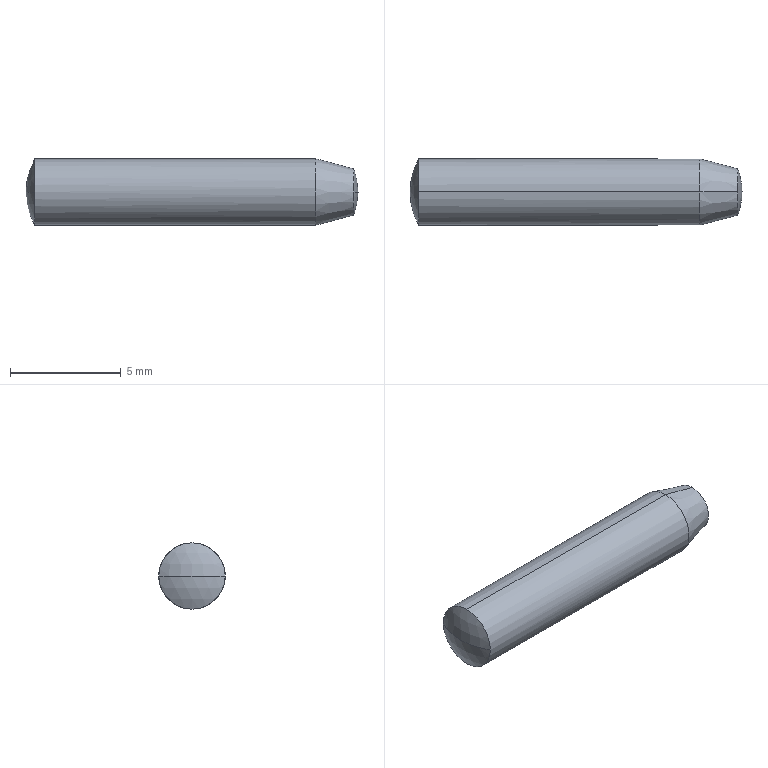Part | NX | features BREP 1 | 1 solid | 8 faces | box 15 x 3 x 3 mm | volume 100.309 mm3 | sphere 4 | cone 2 | cylinder 2 | commonest cylinder face diameters 3 x2
STEP:
#1=CARTESIAN_POINT('',(7.314,-1.04,0.));
#2=VERTEX_POINT('',#1);
#3=CARTESIAN_POINT('',(7.5,0.,0.));
#4=VERTEX_POINT('',#3);
#5=CARTESIAN_POINT('',(4.5,0.,0.));
#6=DIRECTION('',(0.,0.,-1.));
#7=DIRECTION('',(-1.,0.,0.));
#8=AXIS2_PLACEMENT_3D('',#5,#6,#7);
#9=CIRCLE('',#8,3.);
#10=EDGE_CURVE('',#2,#4,#9,.F.);
#11=ORIENTED_EDGE('',*,*,#10,.T.);
#12=CARTESIAN_POINT('',(7.314,1.04,0.));
#13=VERTEX_POINT('',#12);
#14=CARTESIAN_POINT('',(4.5,0.,0.));
#15=DIRECTION('',(0.,0.,1.));
#16=DIRECTION('',(0.,-1.,0.));
#17=AXIS2_PLACEMENT_3D('',#14,#15,#16);
#18=CIRCLE('',#17,3.);
#19=EDGE_CURVE('',#13,#4,#18,.F.);
#20=ORIENTED_EDGE('',*,*,#19,.F.);
#21=CARTESIAN_POINT('',(7.314,0.,1.04));
#22=VERTEX_POINT('',#21);
#23=CARTESIAN_POINT('',(7.314,0.,0.));
#24=DIRECTION('',(-1.,0.,0.));
#25=DIRECTION('',(0.,0.,1.));
#26=AXIS2_PLACEMENT_3D('',#23,#24,#25);
#27=CIRCLE('',#26,1.04);
#28=EDGE_CURVE('',#22,#13,#27,.T.);
#29=ORIENTED_EDGE('',*,*,#28,.F.);
#30=CARTESIAN_POINT('',(7.314,0.,0.));
#31=DIRECTION('',(-1.,0.,0.));
#32=DIRECTION('',(0.,0.,1.));
#33=AXIS2_PLACEMENT_3D('',#30,#31,#32);
#34=CIRCLE('',#33,1.04);
#35=EDGE_CURVE('',#2,#22,#34,.T.);
#36=ORIENTED_EDGE('',*,*,#35,.F.);
#37=EDGE_LOOP('',(#11,#20,#29,#36));
#38=FACE_BOUND('',#37,.T.);
#39=CARTESIAN_POINT('',(4.5,0.,0.));
#40=DIRECTION('',(0.,0.,1.));
#41=DIRECTION('',(0.,1.,0.));
#42=AXIS2_PLACEMENT_3D('',#39,#40,#41);
#43=SPHERICAL_SURFACE('',#42,3.);
#44=ADVANCED_FACE('',(#38),#43,.T.);
#45=ORIENTED_EDGE('',*,*,#28,.T.);
#46=CARTESIAN_POINT('',(7.314,0.,-1.04));
#47=VERTEX_POINT('',#46);
#48=CARTESIAN_POINT('',(7.314,0.,0.));
#49=DIRECTION('',(-1.,0.,0.));
#50=DIRECTION('',(0.,0.,1.));
#51=AXIS2_PLACEMENT_3D('',#48,#49,#50);
#52=CIRCLE('',#51,1.04);
#53=EDGE_CURVE('',#13,#47,#52,.T.);
#54=ORIENTED_EDGE('',*,*,#53,.T.);
#55=CARTESIAN_POINT('',(5.598,0.,-1.5));
#56=VERTEX_POINT('',#55);
#57=CARTESIAN_POINT('',(7.314,0.,-1.04));
#58=DIRECTION('',(-0.9659,0.,-0.2588));
#59=VECTOR('',#58,1000.);
#60=LINE('',#57,#59);
#61=EDGE_CURVE('',#47,#56,#60,.T.);
#62=ORIENTED_EDGE('',*,*,#61,.T.);
#63=CARTESIAN_POINT('',(5.598,0.,1.5));
#64=VERTEX_POINT('',#63);
#65=CARTESIAN_POINT('',(5.598,0.,0.));
#66=DIRECTION('',(-1.,0.,0.));
#67=DIRECTION('',(0.,0.,1.));
#68=AXIS2_PLACEMENT_3D('',#65,#66,#67);
#69=CIRCLE('',#68,1.5);
#70=EDGE_CURVE('',#64,#56,#69,.T.);
#71=ORIENTED_EDGE('',*,*,#70,.F.);
#72=CARTESIAN_POINT('',(7.314,0.,1.04));
#73=DIRECTION('',(-0.9659,0.,0.2588));
#74=VECTOR('',#73,1000.);
#75=LINE('',#72,#74);
#76=EDGE_CURVE('',#22,#64,#75,.T.);
#77=ORIENTED_EDGE('',*,*,#76,.F.);
#78=EDGE_LOOP('',(#45,#54,#62,#71,#77));
#79=FACE_BOUND('',#78,.T.);
#80=CARTESIAN_POINT('',(7.314,0.,0.));
#81=DIRECTION('',(-1.,0.,0.));
#82=DIRECTION('',(0.,0.,-1.));
#83=AXIS2_PLACEMENT_3D('',#80,#81,#82);
#84=CONICAL_SURFACE('',#83,1.04,0.2618);
#85=ADVANCED_FACE('',(#79),#84,.T.);
#86=ORIENTED_EDGE('',*,*,#70,.T.);
#87=CARTESIAN_POINT('',(-7.098,0.,-1.5));
#88=VERTEX_POINT('',#87);
#89=CARTESIAN_POINT('',(7.5,0.,-1.5));
#90=DIRECTION('',(-1.,0.,0.));
#91=VECTOR('',#90,1000.);
#92=LINE('',#89,#91);
#93=EDGE_CURVE('',#56,#88,#92,.T.);
#94=ORIENTED_EDGE('',*,*,#93,.T.);
#95=CARTESIAN_POINT('',(-7.098,1.5,0.));
#96=VERTEX_POINT('',#95);
#97=CARTESIAN_POINT('',(-7.098,0.,0.));
#98=DIRECTION('',(-1.,0.,0.));
#99=DIRECTION('',(0.,0.,1.));
#100=AXIS2_PLACEMENT_3D('',#97,#98,#99);
#101=CIRCLE('',#100,1.5);
#102=EDGE_CURVE('',#96,#88,#101,.T.);
#103=ORIENTED_EDGE('',*,*,#102,.F.);
#104=CARTESIAN_POINT('',(-7.098,0.,1.5));
#105=VERTEX_POINT('',#104);
#106=CARTESIAN_POINT('',(-7.098,0.,0.));
#107=DIRECTION('',(-1.,0.,0.));
#108=DIRECTION('',(0.,0.,1.));
#109=AXIS2_PLACEMENT_3D('',#106,#107,#108);
#110=CIRCLE('',#109,1.5);
#111=EDGE_CURVE('',#105,#96,#110,.T.);
#112=ORIENTED_EDGE('',*,*,#111,.F.);
#113=CARTESIAN_POINT('',(7.5,0.,1.5));
#114=DIRECTION('',(-1.,0.,0.));
#115=VECTOR('',#114,1000.);
#116=LINE('',#113,#115);
#117=EDGE_CURVE('',#64,#105,#116,.T.);
#118=ORIENTED_EDGE('',*,*,#117,.F.);
#119=EDGE_LOOP('',(#86,#94,#103,#112,#118));
#120=FACE_BOUND('',#119,.T.);
#121=CARTESIAN_POINT('',(7.5,0.,0.));
#122=DIRECTION('',(-1.,0.,0.));
#123=DIRECTION('',(0.,0.,-1.));
#124=AXIS2_PLACEMENT_3D('',#121,#122,#123);
#125=CYLINDRICAL_SURFACE('',#124,1.5);
#126=ADVANCED_FACE('',(#120),#125,.T.);
#127=ORIENTED_EDGE('',*,*,#102,.T.);
#128=CARTESIAN_POINT('',(-7.098,-1.5,0.));
#129=VERTEX_POINT('',#128);
#130=CARTESIAN_POINT('',(-7.098,0.,0.));
#131=DIRECTION('',(-1.,0.,0.));
#132=DIRECTION('',(0.,0.,1.));
#133=AXIS2_PLACEMENT_3D('',#130,#131,#132);
#134=CIRCLE('',#133,1.5);
#135=EDGE_CURVE('',#88,#129,#134,.T.);
#136=ORIENTED_EDGE('',*,*,#135,.T.);
#137=CARTESIAN_POINT('',(-7.5,0.,0.));
#138=VERTEX_POINT('',#137);
#139=CARTESIAN_POINT('',(-4.5,0.,0.));
#140=DIRECTION('',(0.,0.,-1.));
#141=DIRECTION('',(0.,1.,0.));
#142=AXIS2_PLACEMENT_3D('',#139,#140,#141);
#143=CIRCLE('',#142,3.);
#144=EDGE_CURVE('',#129,#138,#143,.T.);
#145=ORIENTED_EDGE('',*,*,#144,.T.);
#146=CARTESIAN_POINT('',(-4.5,0.,0.));
#147=DIRECTION('',(0.,0.,1.));
#148=DIRECTION('',(1.,0.,0.));
#149=AXIS2_PLACEMENT_3D('',#146,#147,#148);
#150=CIRCLE('',#149,3.);
#151=EDGE_CURVE('',#96,#138,#150,.T.);
#152=ORIENTED_EDGE('',*,*,#151,.F.);
#153=EDGE_LOOP('',(#127,#136,#145,#152));
#154=FACE_BOUND('',#153,.T.);
#155=CARTESIAN_POINT('',(-4.5,0.,0.));
#156=DIRECTION('',(0.,0.,-1.));
#157=DIRECTION('',(0.,-1.,0.));
#158=AXIS2_PLACEMENT_3D('',#155,#156,#157);
#159=SPHERICAL_SURFACE('',#158,3.);
#160=ADVANCED_FACE('',(#154),#159,.T.);
#161=ORIENTED_EDGE('',*,*,#144,.F.);
#162=CARTESIAN_POINT('',(-7.098,0.,0.));
#163=DIRECTION('',(-1.,0.,0.));
#164=DIRECTION('',(0.,0.,1.));
#165=AXIS2_PLACEMENT_3D('',#162,#163,#164);
#166=CIRCLE('',#165,1.5);
#167=EDGE_CURVE('',#129,#105,#166,.T.);
#168=ORIENTED_EDGE('',*,*,#167,.T.);
#169=ORIENTED_EDGE('',*,*,#111,.T.);
#170=ORIENTED_EDGE('',*,*,#151,.T.);
#171=EDGE_LOOP('',(#161,#168,#169,#170));
#172=FACE_BOUND('',#171,.T.);
#173=CARTESIAN_POINT('',(-4.5,0.,0.));
#174=DIRECTION('',(0.,0.,-1.));
#175=DIRECTION('',(0.,-1.,0.));
#176=AXIS2_PLACEMENT_3D('',#173,#174,#175);
#177=SPHERICAL_SURFACE('',#176,3.);
#178=ADVANCED_FACE('',(#172),#177,.T.);
#179=ORIENTED_EDGE('',*,*,#93,.F.);
#180=CARTESIAN_POINT('',(5.598,0.,0.));
#181=DIRECTION('',(-1.,0.,0.));
#182=DIRECTION('',(0.,0.,1.));
#183=AXIS2_PLACEMENT_3D('',#180,#181,#182);
#184=CIRCLE('',#183,1.5);
#185=EDGE_CURVE('',#56,#64,#184,.T.);
#186=ORIENTED_EDGE('',*,*,#185,.T.);
#187=ORIENTED_EDGE('',*,*,#117,.T.);
#188=ORIENTED_EDGE('',*,*,#167,.F.);
#189=ORIENTED_EDGE('',*,*,#135,.F.);
#190=EDGE_LOOP('',(#179,#186,#187,#188,#189));
#191=FACE_BOUND('',#190,.T.);
#192=CARTESIAN_POINT('',(7.5,0.,0.));
#193=DIRECTION('',(-1.,0.,0.));
#194=DIRECTION('',(0.,0.,-1.));
#195=AXIS2_PLACEMENT_3D('',#192,#193,#194);
#196=CYLINDRICAL_SURFACE('',#195,1.5);
#197=ADVANCED_FACE('',(#191),#196,.T.);
#198=ORIENTED_EDGE('',*,*,#61,.F.);
#199=CARTESIAN_POINT('',(7.314,0.,0.));
#200=DIRECTION('',(-1.,0.,0.));
#201=DIRECTION('',(0.,0.,1.));
#202=AXIS2_PLACEMENT_3D('',#199,#200,#201);
#203=CIRCLE('',#202,1.04);
#204=EDGE_CURVE('',#47,#2,#203,.T.);
#205=ORIENTED_EDGE('',*,*,#204,.T.);
#206=ORIENTED_EDGE('',*,*,#35,.T.);
#207=ORIENTED_EDGE('',*,*,#76,.T.);
#208=ORIENTED_EDGE('',*,*,#185,.F.);
#209=EDGE_LOOP('',(#198,#205,#206,#207,#208));
#210=FACE_BOUND('',#209,.T.);
#211=CARTESIAN_POINT('',(7.314,0.,0.));
#212=DIRECTION('',(-1.,0.,0.));
#213=DIRECTION('',(0.,0.,-1.));
#214=AXIS2_PLACEMENT_3D('',#211,#212,#213);
#215=CONICAL_SURFACE('',#214,1.04,0.2618);
#216=ADVANCED_FACE('',(#210),#215,.T.);
#217=ORIENTED_EDGE('',*,*,#19,.T.);
#218=ORIENTED_EDGE('',*,*,#10,.F.);
#219=ORIENTED_EDGE('',*,*,#204,.F.);
#220=ORIENTED_EDGE('',*,*,#53,.F.);
#221=EDGE_LOOP('',(#217,#218,#219,#220));
#222=FACE_BOUND('',#221,.T.);
#223=CARTESIAN_POINT('',(4.5,0.,0.));
#224=DIRECTION('',(0.,0.,1.));
#225=DIRECTION('',(0.,1.,0.));
#226=AXIS2_PLACEMENT_3D('',#223,#224,#225);
#227=SPHERICAL_SURFACE('',#226,3.);
#228=ADVANCED_FACE('',(#222),#227,.T.);
#229=CLOSED_SHELL('',(#44,#85,#126,#160,#178,#197,#216,#228));
#230=MANIFOLD_SOLID_BREP('',#229);
#231=(LENGTH_UNIT()NAMED_UNIT(*)SI_UNIT(.MILLI.,.METRE.));
#232=UNCERTAINTY_MEASURE_WITH_UNIT(LENGTH_MEASURE(0.00001),#231,'','');
#233=(NAMED_UNIT(*)PLANE_ANGLE_UNIT()SI_UNIT($,.RADIAN.));
#234=(NAMED_UNIT(*)SI_UNIT($,.STERADIAN.)SOLID_ANGLE_UNIT());
#235=(GEOMETRIC_REPRESENTATION_CONTEXT(3)GLOBAL_UNCERTAINTY_ASSIGNED_CONTEXT((#232))GLOBAL_UNIT_ASSIGNED_CONTEXT((#231,#233,#234))REPRESENTATION_CONTEXT('',''));
#236=ADVANCED_BREP_SHAPE_REPRESENTATION('',(#230),#235);